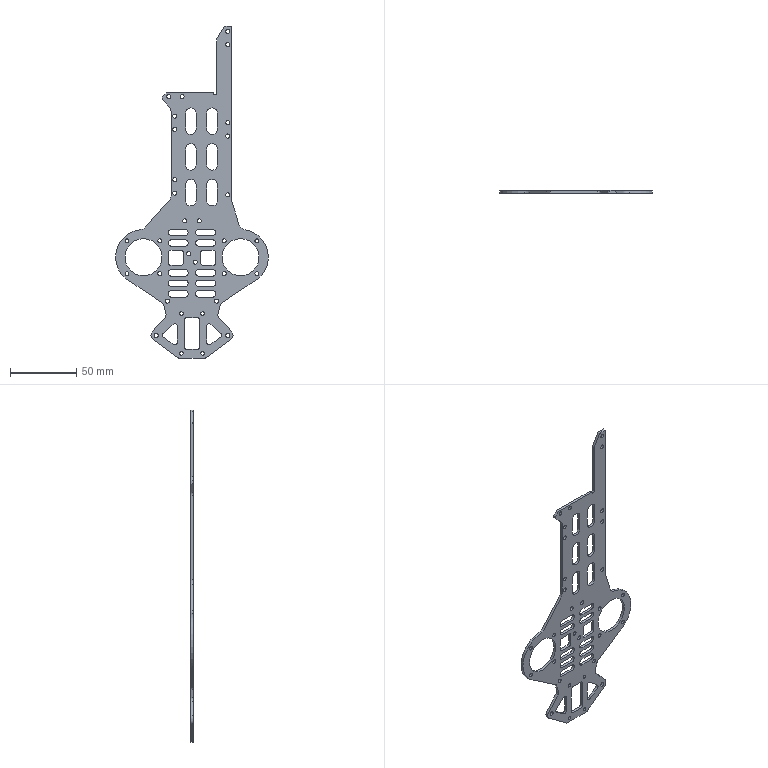Part | SolidWorks | features Fillet 3, ICE 2, Chamfer 1, Extrusion 1 | 1 solid | 214 faces | box 115.25 x 2 x 250.4 mm | volume 18165 mm3 | cylinder 142 | plane 72 | commonest cylinder face diameters 3.1 x34 4 x24 5 x20 8 x20 3 x16 2.65 x8